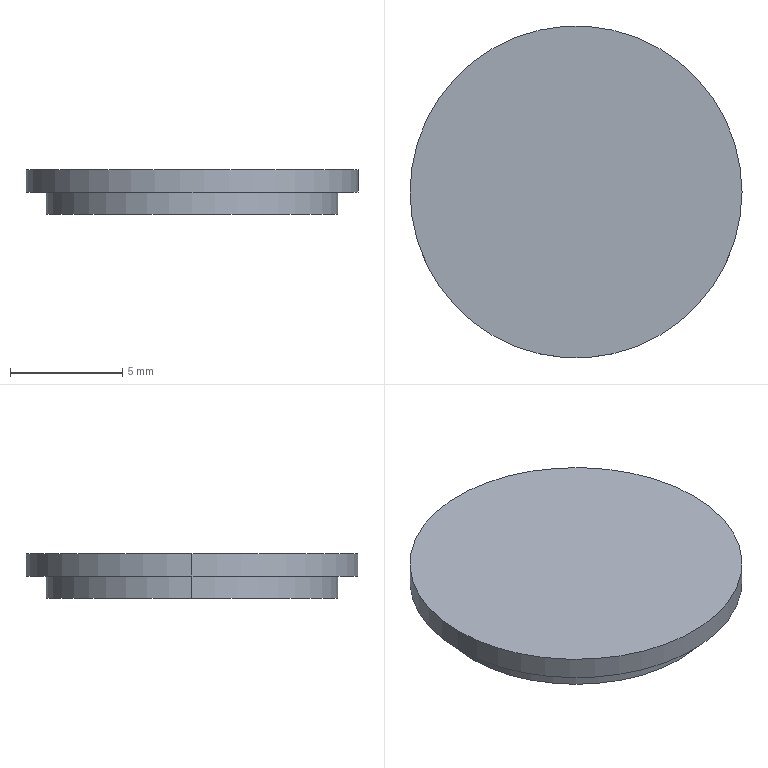Part | SolidWorks | features Extrusion 1, ICE 1 | 1 solid | 7 faces | box 14.8 x 14.8 x 2 mm | volume 304.766 mm3 | cylinder 4 | plane 3 | commonest cylinder face diameters 13 x2 14.8 x2
STEP:
#1=CARTESIAN_POINT('',(6.5,0.,-1.));
#2=VERTEX_POINT('',#1);
#3=CARTESIAN_POINT('',(-6.5,0.,-1.));
#4=VERTEX_POINT('',#3);
#5=CARTESIAN_POINT('',(0.,0.,-1.));
#6=DIRECTION('',(0.,0.,1.));
#7=DIRECTION('',(1.,0.,0.));
#8=AXIS2_PLACEMENT_3D('',#5,#6,#7);
#9=CIRCLE('',#8,6.5);
#10=EDGE_CURVE('',#2,#4,#9,.T.);
#11=ORIENTED_EDGE('',*,*,#10,.T.);
#12=CARTESIAN_POINT('',(-6.5,0.,0.));
#13=VERTEX_POINT('',#12);
#14=CARTESIAN_POINT('',(-6.5,0.,-1.));
#15=DIRECTION('',(0.,0.,1.));
#16=VECTOR('',#15,1000.);
#17=LINE('',#14,#16);
#18=EDGE_CURVE('',#4,#13,#17,.T.);
#19=ORIENTED_EDGE('',*,*,#18,.T.);
#20=CARTESIAN_POINT('',(6.5,0.,0.));
#21=VERTEX_POINT('',#20);
#22=CARTESIAN_POINT('',(0.,0.,0.));
#23=DIRECTION('',(0.,0.,1.));
#24=DIRECTION('',(1.,0.,0.));
#25=AXIS2_PLACEMENT_3D('',#22,#23,#24);
#26=CIRCLE('',#25,6.5);
#27=EDGE_CURVE('',#21,#13,#26,.T.);
#28=ORIENTED_EDGE('',*,*,#27,.F.);
#29=CARTESIAN_POINT('',(6.5,0.,-1.));
#30=DIRECTION('',(0.,0.,1.));
#31=VECTOR('',#30,1000.);
#32=LINE('',#29,#31);
#33=EDGE_CURVE('',#2,#21,#32,.T.);
#34=ORIENTED_EDGE('',*,*,#33,.F.);
#35=EDGE_LOOP('',(#11,#19,#28,#34));
#36=FACE_OUTER_BOUND('',#35,.T.);
#37=CARTESIAN_POINT('',(0.,0.,-1.));
#38=DIRECTION('',(0.,0.,1.));
#39=DIRECTION('',(1.,0.,0.));
#40=AXIS2_PLACEMENT_3D('',#37,#38,#39);
#41=CYLINDRICAL_SURFACE('',#40,6.5);
#42=ADVANCED_FACE('',(#36),#41,.T.);
#43=CARTESIAN_POINT('',(7.4,0.,1.));
#44=VERTEX_POINT('',#43);
#45=CARTESIAN_POINT('',(-7.4,0.,1.));
#46=VERTEX_POINT('',#45);
#47=CARTESIAN_POINT('',(0.,0.,1.));
#48=DIRECTION('',(0.,0.,1.));
#49=DIRECTION('',(1.,0.,0.));
#50=AXIS2_PLACEMENT_3D('',#47,#48,#49);
#51=CIRCLE('',#50,7.4);
#52=EDGE_CURVE('',#44,#46,#51,.T.);
#53=ORIENTED_EDGE('',*,*,#52,.F.);
#54=CARTESIAN_POINT('',(7.4,0.,0.));
#55=VERTEX_POINT('',#54);
#56=CARTESIAN_POINT('',(7.4,0.,1.));
#57=DIRECTION('',(0.,0.,-1.));
#58=VECTOR('',#57,1000.);
#59=LINE('',#56,#58);
#60=EDGE_CURVE('',#44,#55,#59,.T.);
#61=ORIENTED_EDGE('',*,*,#60,.T.);
#62=CARTESIAN_POINT('',(-7.4,0.,0.));
#63=VERTEX_POINT('',#62);
#64=CARTESIAN_POINT('',(0.,0.,0.));
#65=DIRECTION('',(0.,0.,1.));
#66=DIRECTION('',(1.,0.,0.));
#67=AXIS2_PLACEMENT_3D('',#64,#65,#66);
#68=CIRCLE('',#67,7.4);
#69=EDGE_CURVE('',#55,#63,#68,.T.);
#70=ORIENTED_EDGE('',*,*,#69,.T.);
#71=CARTESIAN_POINT('',(-7.4,0.,1.));
#72=DIRECTION('',(0.,0.,-1.));
#73=VECTOR('',#72,1000.);
#74=LINE('',#71,#73);
#75=EDGE_CURVE('',#46,#63,#74,.T.);
#76=ORIENTED_EDGE('',*,*,#75,.F.);
#77=EDGE_LOOP('',(#53,#61,#70,#76));
#78=FACE_OUTER_BOUND('',#77,.T.);
#79=CARTESIAN_POINT('',(0.,0.,1.));
#80=DIRECTION('',(0.,0.,-1.));
#81=DIRECTION('',(-1.,0.,0.));
#82=AXIS2_PLACEMENT_3D('',#79,#80,#81);
#83=CYLINDRICAL_SURFACE('',#82,7.4);
#84=ADVANCED_FACE('',(#78),#83,.T.);
#85=ORIENTED_EDGE('',*,*,#60,.F.);
#86=CARTESIAN_POINT('',(0.,0.,1.));
#87=DIRECTION('',(0.,0.,1.));
#88=DIRECTION('',(1.,0.,0.));
#89=AXIS2_PLACEMENT_3D('',#86,#87,#88);
#90=CIRCLE('',#89,7.4);
#91=EDGE_CURVE('',#46,#44,#90,.T.);
#92=ORIENTED_EDGE('',*,*,#91,.F.);
#93=ORIENTED_EDGE('',*,*,#75,.T.);
#94=CARTESIAN_POINT('',(0.,0.,0.));
#95=DIRECTION('',(0.,0.,1.));
#96=DIRECTION('',(1.,0.,0.));
#97=AXIS2_PLACEMENT_3D('',#94,#95,#96);
#98=CIRCLE('',#97,7.4);
#99=EDGE_CURVE('',#63,#55,#98,.T.);
#100=ORIENTED_EDGE('',*,*,#99,.T.);
#101=EDGE_LOOP('',(#85,#92,#93,#100));
#102=FACE_OUTER_BOUND('',#101,.T.);
#103=CARTESIAN_POINT('',(0.,0.,1.));
#104=DIRECTION('',(0.,0.,-1.));
#105=DIRECTION('',(-1.,0.,0.));
#106=AXIS2_PLACEMENT_3D('',#103,#104,#105);
#107=CYLINDRICAL_SURFACE('',#106,7.4);
#108=ADVANCED_FACE('',(#102),#107,.T.);
#109=ORIENTED_EDGE('',*,*,#91,.T.);
#110=ORIENTED_EDGE('',*,*,#52,.T.);
#111=EDGE_LOOP('',(#109,#110));
#112=FACE_OUTER_BOUND('',#111,.T.);
#113=CARTESIAN_POINT('',(0.,0.,1.));
#114=DIRECTION('',(0.,0.,1.));
#115=DIRECTION('',(1.,0.,0.));
#116=AXIS2_PLACEMENT_3D('',#113,#114,#115);
#117=PLANE('',#116);
#118=ADVANCED_FACE('',(#112),#117,.T.);
#119=ORIENTED_EDGE('',*,*,#27,.T.);
#120=CARTESIAN_POINT('',(0.,0.,0.));
#121=DIRECTION('',(0.,0.,1.));
#122=DIRECTION('',(1.,0.,0.));
#123=AXIS2_PLACEMENT_3D('',#120,#121,#122);
#124=CIRCLE('',#123,6.5);
#125=EDGE_CURVE('',#13,#21,#124,.T.);
#126=ORIENTED_EDGE('',*,*,#125,.T.);
#127=EDGE_LOOP('',(#119,#126));
#128=FACE_BOUND('',#127,.T.);
#129=ORIENTED_EDGE('',*,*,#99,.F.);
#130=ORIENTED_EDGE('',*,*,#69,.F.);
#131=EDGE_LOOP('',(#129,#130));
#132=FACE_OUTER_BOUND('',#131,.T.);
#133=CARTESIAN_POINT('',(0.,0.,0.));
#134=DIRECTION('',(0.,0.,1.));
#135=DIRECTION('',(1.,0.,0.));
#136=AXIS2_PLACEMENT_3D('',#133,#134,#135);
#137=PLANE('',#136);
#138=ADVANCED_FACE('',(#128,#132),#137,.F.);
#139=ORIENTED_EDGE('',*,*,#18,.F.);
#140=CARTESIAN_POINT('',(0.,0.,-1.));
#141=DIRECTION('',(0.,0.,1.));
#142=DIRECTION('',(1.,0.,0.));
#143=AXIS2_PLACEMENT_3D('',#140,#141,#142);
#144=CIRCLE('',#143,6.5);
#145=EDGE_CURVE('',#4,#2,#144,.T.);
#146=ORIENTED_EDGE('',*,*,#145,.T.);
#147=ORIENTED_EDGE('',*,*,#33,.T.);
#148=ORIENTED_EDGE('',*,*,#125,.F.);
#149=EDGE_LOOP('',(#139,#146,#147,#148));
#150=FACE_OUTER_BOUND('',#149,.T.);
#151=CARTESIAN_POINT('',(0.,0.,-1.));
#152=DIRECTION('',(0.,0.,1.));
#153=DIRECTION('',(1.,0.,0.));
#154=AXIS2_PLACEMENT_3D('',#151,#152,#153);
#155=CYLINDRICAL_SURFACE('',#154,6.5);
#156=ADVANCED_FACE('',(#150),#155,.T.);
#157=ORIENTED_EDGE('',*,*,#10,.F.);
#158=ORIENTED_EDGE('',*,*,#145,.F.);
#159=EDGE_LOOP('',(#157,#158));
#160=FACE_OUTER_BOUND('',#159,.T.);
#161=CARTESIAN_POINT('',(0.,0.,-1.));
#162=DIRECTION('',(0.,0.,1.));
#163=DIRECTION('',(1.,0.,0.));
#164=AXIS2_PLACEMENT_3D('',#161,#162,#163);
#165=PLANE('',#164);
#166=ADVANCED_FACE('',(#160),#165,.F.);
#167=CLOSED_SHELL('',(#42,#84,#108,#118,#138,#156,#166));
#168=MANIFOLD_SOLID_BREP('',#167);
#169=CARTESIAN_POINT('',(0.,0.,0.));
#170=DIRECTION('',(0.,0.,1.));
#171=DIRECTION('',(1.,0.,0.));
#172=AXIS2_PLACEMENT_3D('',#169,#170,#171);
#173=(LENGTH_UNIT()NAMED_UNIT(*)SI_UNIT(.MILLI.,.METRE.));
#174=UNCERTAINTY_MEASURE_WITH_UNIT(LENGTH_MEASURE(0.00001),#173,'','');
#175=(NAMED_UNIT(*)PLANE_ANGLE_UNIT()SI_UNIT($,.RADIAN.));
#176=(NAMED_UNIT(*)SI_UNIT($,.STERADIAN.)SOLID_ANGLE_UNIT());
#177=(GEOMETRIC_REPRESENTATION_CONTEXT(3)GLOBAL_UNCERTAINTY_ASSIGNED_CONTEXT((#174))GLOBAL_UNIT_ASSIGNED_CONTEXT((#173,#175,#176))REPRESENTATION_CONTEXT('',''));
#178=ADVANCED_BREP_SHAPE_REPRESENTATION('',(#168,#172),#177);